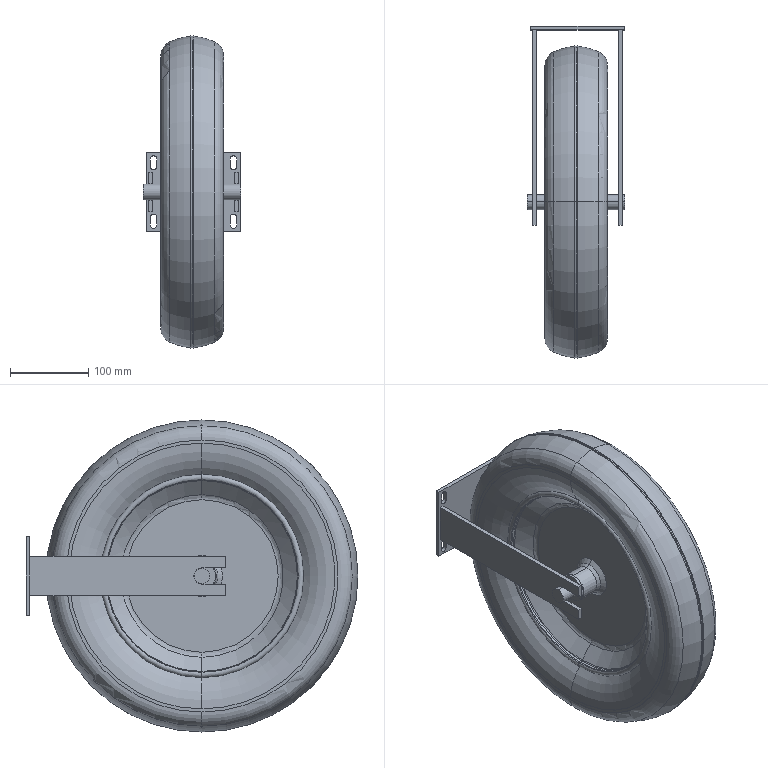Part | SolidWorks | 3 solids | 208 faces | box 125 x 424.531 x 399.062 mm | volume 1072576 mm3 | torus 72 | cylinder 52 | plane 48 | cone 36 | commonest cylinder face diameters 8.258 x12 20 x6 33.4 x4 35 x4 36.4 x4 245.5 x4